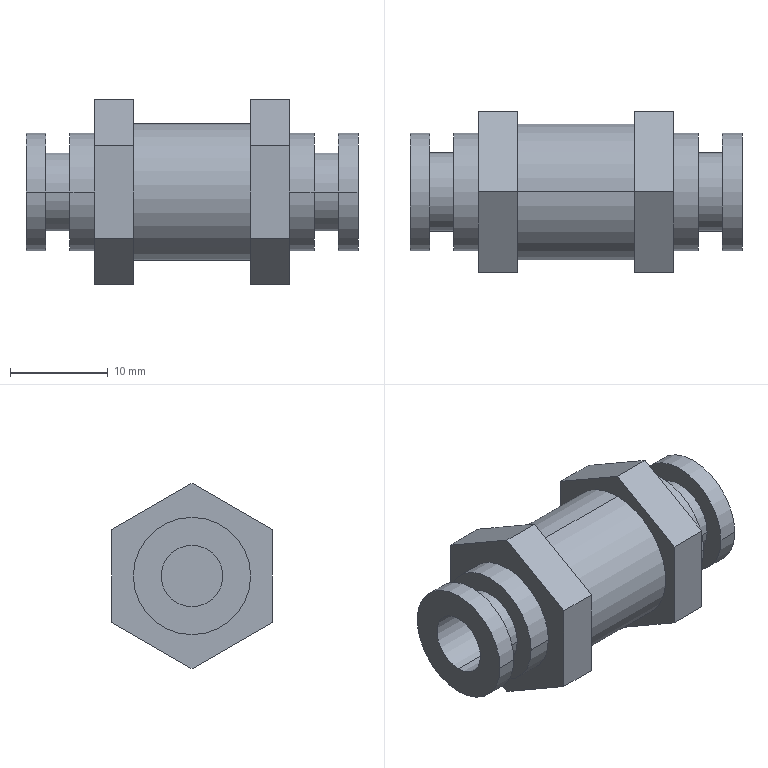Part | STEP file | QIGUANJIEKOU.stp.STEP | 1 solid | 42 faces | box 34 x 16.454 x 19 mm | volume 4306 mm3 | plane 24 | cylinder 18 | commonest cylinder face diameters 12 x8 6.3 x4 8 x4 14 x2
STEP:
#1=CARTESIAN_POINT('',(17.,0.,-3.15));
#2=VERTEX_POINT('',#1);
#3=CARTESIAN_POINT('',(17.,0.,3.15));
#4=VERTEX_POINT('',#3);
#5=CARTESIAN_POINT('',(17.,0.,0.));
#6=DIRECTION('',(1.,0.,0.));
#7=DIRECTION('',(0.,0.,-1.));
#8=AXIS2_PLACEMENT_3D('',#5,#6,#7);
#9=CIRCLE('',#8,3.15);
#10=EDGE_CURVE('',#2,#4,#9,.T.);
#11=ORIENTED_EDGE('',*,*,#10,.F.);
#12=CARTESIAN_POINT('',(17.,0.,0.));
#13=DIRECTION('',(1.,0.,0.));
#14=DIRECTION('',(0.,0.,1.));
#15=AXIS2_PLACEMENT_3D('',#12,#13,#14);
#16=CIRCLE('',#15,3.15);
#17=EDGE_CURVE('',#4,#2,#16,.T.);
#18=ORIENTED_EDGE('',*,*,#17,.F.);
#19=EDGE_LOOP('',(#11,#18));
#20=FACE_BOUND('',#19,.T.);
#21=CARTESIAN_POINT('',(17.,6.,0.));
#22=VERTEX_POINT('',#21);
#23=CARTESIAN_POINT('',(17.,-6.,0.));
#24=VERTEX_POINT('',#23);
#25=CARTESIAN_POINT('',(17.,0.,0.));
#26=DIRECTION('',(1.,0.,0.));
#27=DIRECTION('',(0.,1.,0.));
#28=AXIS2_PLACEMENT_3D('',#25,#26,#27);
#29=CIRCLE('',#28,6.);
#30=EDGE_CURVE('',#22,#24,#29,.T.);
#31=ORIENTED_EDGE('',*,*,#30,.T.);
#32=CARTESIAN_POINT('',(17.,0.,0.));
#33=DIRECTION('',(-1.,0.,0.));
#34=DIRECTION('',(0.,1.,0.));
#35=AXIS2_PLACEMENT_3D('',#32,#33,#34);
#36=CIRCLE('',#35,6.);
#37=EDGE_CURVE('',#22,#24,#36,.T.);
#38=ORIENTED_EDGE('',*,*,#37,.F.);
#39=EDGE_LOOP('',(#31,#38));
#40=FACE_OUTER_BOUND('',#39,.T.);
#41=CARTESIAN_POINT('',(17.,0.,0.));
#42=DIRECTION('',(1.,0.,0.));
#43=DIRECTION('',(0.,1.,0.));
#44=AXIS2_PLACEMENT_3D('',#41,#42,#43);
#45=PLANE('',#44);
#46=ADVANCED_FACE('',(#20,#40),#45,.T.);
#47=CARTESIAN_POINT('',(15.,6.,0.));
#48=VERTEX_POINT('',#47);
#49=CARTESIAN_POINT('',(17.,6.,0.));
#50=DIRECTION('',(-1.,0.,0.));
#51=VECTOR('',#50,1000.);
#52=LINE('',#49,#51);
#53=EDGE_CURVE('',#22,#48,#52,.T.);
#54=ORIENTED_EDGE('',*,*,#53,.F.);
#55=ORIENTED_EDGE('',*,*,#37,.T.);
#56=CARTESIAN_POINT('',(15.,-6.,0.));
#57=VERTEX_POINT('',#56);
#58=CARTESIAN_POINT('',(17.,-6.,0.));
#59=DIRECTION('',(-1.,0.,0.));
#60=VECTOR('',#59,1000.);
#61=LINE('',#58,#60);
#62=EDGE_CURVE('',#24,#57,#61,.T.);
#63=ORIENTED_EDGE('',*,*,#62,.T.);
#64=CARTESIAN_POINT('',(15.,0.,0.));
#65=DIRECTION('',(1.,0.,0.));
#66=DIRECTION('',(0.,-1.,0.));
#67=AXIS2_PLACEMENT_3D('',#64,#65,#66);
#68=CIRCLE('',#67,6.);
#69=EDGE_CURVE('',#57,#48,#68,.T.);
#70=ORIENTED_EDGE('',*,*,#69,.T.);
#71=EDGE_LOOP('',(#54,#55,#63,#70));
#72=FACE_OUTER_BOUND('',#71,.T.);
#73=CARTESIAN_POINT('',(-18.7,0.,0.));
#74=DIRECTION('',(1.,0.,0.));
#75=DIRECTION('',(0.,-1.,0.));
#76=AXIS2_PLACEMENT_3D('',#73,#74,#75);
#77=CYLINDRICAL_SURFACE('',#76,6.);
#78=ADVANCED_FACE('',(#72),#77,.T.);
#79=CARTESIAN_POINT('',(12.5,-6.,0.));
#80=VERTEX_POINT('',#79);
#81=CARTESIAN_POINT('',(10.,-6.,0.));
#82=VERTEX_POINT('',#81);
#83=CARTESIAN_POINT('',(12.5,-6.,0.));
#84=DIRECTION('',(-1.,0.,0.));
#85=VECTOR('',#84,1000.);
#86=LINE('',#83,#85);
#87=EDGE_CURVE('',#80,#82,#86,.T.);
#88=ORIENTED_EDGE('',*,*,#87,.T.);
#89=CARTESIAN_POINT('',(10.,6.,0.));
#90=VERTEX_POINT('',#89);
#91=CARTESIAN_POINT('',(10.,0.,0.));
#92=DIRECTION('',(-1.,0.,0.));
#93=DIRECTION('',(0.,1.,0.));
#94=AXIS2_PLACEMENT_3D('',#91,#92,#93);
#95=CIRCLE('',#94,6.);
#96=EDGE_CURVE('',#90,#82,#95,.T.);
#97=ORIENTED_EDGE('',*,*,#96,.F.);
#98=CARTESIAN_POINT('',(12.5,6.,0.));
#99=VERTEX_POINT('',#98);
#100=CARTESIAN_POINT('',(12.5,6.,0.));
#101=DIRECTION('',(-1.,0.,0.));
#102=VECTOR('',#101,1000.);
#103=LINE('',#100,#102);
#104=EDGE_CURVE('',#99,#90,#103,.T.);
#105=ORIENTED_EDGE('',*,*,#104,.F.);
#106=CARTESIAN_POINT('',(12.5,0.,0.));
#107=DIRECTION('',(1.,0.,0.));
#108=DIRECTION('',(0.,-1.,0.));
#109=AXIS2_PLACEMENT_3D('',#106,#107,#108);
#110=CIRCLE('',#109,6.);
#111=EDGE_CURVE('',#80,#99,#110,.T.);
#112=ORIENTED_EDGE('',*,*,#111,.F.);
#113=EDGE_LOOP('',(#88,#97,#105,#112));
#114=FACE_OUTER_BOUND('',#113,.T.);
#115=CARTESIAN_POINT('',(-18.7,0.,0.));
#116=DIRECTION('',(1.,0.,0.));
#117=DIRECTION('',(0.,-1.,0.));
#118=AXIS2_PLACEMENT_3D('',#115,#116,#117);
#119=CYLINDRICAL_SURFACE('',#118,6.);
#120=ADVANCED_FACE('',(#114),#119,.T.);
#121=CARTESIAN_POINT('',(-15.,-6.,0.));
#122=VERTEX_POINT('',#121);
#123=CARTESIAN_POINT('',(-17.,-6.,0.));
#124=VERTEX_POINT('',#123);
#125=CARTESIAN_POINT('',(-15.,-6.,0.));
#126=DIRECTION('',(-1.,0.,0.));
#127=VECTOR('',#126,1000.);
#128=LINE('',#125,#127);
#129=EDGE_CURVE('',#122,#124,#128,.T.);
#130=ORIENTED_EDGE('',*,*,#129,.T.);
#131=CARTESIAN_POINT('',(-17.,6.,0.));
#132=VERTEX_POINT('',#131);
#133=CARTESIAN_POINT('',(-17.,0.,0.));
#134=DIRECTION('',(-1.,0.,0.));
#135=DIRECTION('',(0.,1.,0.));
#136=AXIS2_PLACEMENT_3D('',#133,#134,#135);
#137=CIRCLE('',#136,6.);
#138=EDGE_CURVE('',#132,#124,#137,.T.);
#139=ORIENTED_EDGE('',*,*,#138,.F.);
#140=CARTESIAN_POINT('',(-15.,6.,0.));
#141=VERTEX_POINT('',#140);
#142=CARTESIAN_POINT('',(-15.,6.,0.));
#143=DIRECTION('',(-1.,0.,0.));
#144=VECTOR('',#143,1000.);
#145=LINE('',#142,#144);
#146=EDGE_CURVE('',#141,#132,#145,.T.);
#147=ORIENTED_EDGE('',*,*,#146,.F.);
#148=CARTESIAN_POINT('',(-15.,0.,0.));
#149=DIRECTION('',(1.,0.,0.));
#150=DIRECTION('',(0.,-1.,0.));
#151=AXIS2_PLACEMENT_3D('',#148,#149,#150);
#152=CIRCLE('',#151,6.);
#153=EDGE_CURVE('',#122,#141,#152,.T.);
#154=ORIENTED_EDGE('',*,*,#153,.F.);
#155=EDGE_LOOP('',(#130,#139,#147,#154));
#156=FACE_OUTER_BOUND('',#155,.T.);
#157=CARTESIAN_POINT('',(-18.7,0.,0.));
#158=DIRECTION('',(1.,0.,0.));
#159=DIRECTION('',(0.,-1.,0.));
#160=AXIS2_PLACEMENT_3D('',#157,#158,#159);
#161=CYLINDRICAL_SURFACE('',#160,6.);
#162=ADVANCED_FACE('',(#156),#161,.T.);
#163=CARTESIAN_POINT('',(-10.,6.,0.));
#164=VERTEX_POINT('',#163);
#165=CARTESIAN_POINT('',(-12.5,6.,0.));
#166=VERTEX_POINT('',#165);
#167=CARTESIAN_POINT('',(-10.,6.,0.));
#168=DIRECTION('',(-1.,0.,0.));
#169=VECTOR('',#168,1000.);
#170=LINE('',#167,#169);
#171=EDGE_CURVE('',#164,#166,#170,.T.);
#172=ORIENTED_EDGE('',*,*,#171,.F.);
#173=CARTESIAN_POINT('',(-10.,-6.,0.));
#174=VERTEX_POINT('',#173);
#175=CARTESIAN_POINT('',(-10.,0.,0.));
#176=DIRECTION('',(1.,0.,0.));
#177=DIRECTION('',(0.,-1.,0.));
#178=AXIS2_PLACEMENT_3D('',#175,#176,#177);
#179=CIRCLE('',#178,6.);
#180=EDGE_CURVE('',#174,#164,#179,.T.);
#181=ORIENTED_EDGE('',*,*,#180,.F.);
#182=CARTESIAN_POINT('',(-12.5,-6.,0.));
#183=VERTEX_POINT('',#182);
#184=CARTESIAN_POINT('',(-10.,-6.,0.));
#185=DIRECTION('',(-1.,0.,0.));
#186=VECTOR('',#185,1000.);
#187=LINE('',#184,#186);
#188=EDGE_CURVE('',#174,#183,#187,.T.);
#189=ORIENTED_EDGE('',*,*,#188,.T.);
#190=CARTESIAN_POINT('',(-12.5,0.,0.));
#191=DIRECTION('',(1.,0.,0.));
#192=DIRECTION('',(0.,-1.,0.));
#193=AXIS2_PLACEMENT_3D('',#190,#191,#192);
#194=CIRCLE('',#193,6.);
#195=EDGE_CURVE('',#183,#166,#194,.T.);
#196=ORIENTED_EDGE('',*,*,#195,.T.);
#197=EDGE_LOOP('',(#172,#181,#189,#196));
#198=FACE_OUTER_BOUND('',#197,.T.);
#199=CARTESIAN_POINT('',(-18.7,0.,0.));
#200=DIRECTION('',(1.,0.,0.));
#201=DIRECTION('',(0.,-1.,0.));
#202=AXIS2_PLACEMENT_3D('',#199,#200,#201);
#203=CYLINDRICAL_SURFACE('',#202,6.);
#204=ADVANCED_FACE('',(#198),#203,.T.);
#205=CARTESIAN_POINT('',(15.,-4.,0.));
#206=VERTEX_POINT('',#205);
#207=CARTESIAN_POINT('',(15.,4.,0.));
#208=VERTEX_POINT('',#207);
#209=CARTESIAN_POINT('',(15.,0.,0.));
#210=DIRECTION('',(1.,0.,0.));
#211=DIRECTION('',(0.,-1.,0.));
#212=AXIS2_PLACEMENT_3D('',#209,#210,#211);
#213=CIRCLE('',#212,4.);
#214=EDGE_CURVE('',#206,#208,#213,.T.);
#215=ORIENTED_EDGE('',*,*,#214,.T.);
#216=CARTESIAN_POINT('',(15.,0.,0.));
#217=DIRECTION('',(-1.,0.,0.));
#218=DIRECTION('',(0.,-1.,0.));
#219=AXIS2_PLACEMENT_3D('',#216,#217,#218);
#220=CIRCLE('',#219,4.);
#221=EDGE_CURVE('',#206,#208,#220,.T.);
#222=ORIENTED_EDGE('',*,*,#221,.F.);
#223=EDGE_LOOP('',(#215,#222));
#224=FACE_BOUND('',#223,.T.);
#225=ORIENTED_EDGE('',*,*,#69,.F.);
#226=CARTESIAN_POINT('',(15.,0.,0.));
#227=DIRECTION('',(1.,0.,0.));
#228=DIRECTION('',(0.,1.,0.));
#229=AXIS2_PLACEMENT_3D('',#226,#227,#228);
#230=CIRCLE('',#229,6.);
#231=EDGE_CURVE('',#48,#57,#230,.T.);
#232=ORIENTED_EDGE('',*,*,#231,.F.);
#233=EDGE_LOOP('',(#225,#232));
#234=FACE_OUTER_BOUND('',#233,.T.);
#235=CARTESIAN_POINT('',(15.,0.,0.));
#236=DIRECTION('',(1.,0.,0.));
#237=DIRECTION('',(0.,1.,0.));
#238=AXIS2_PLACEMENT_3D('',#235,#236,#237);
#239=PLANE('',#238);
#240=ADVANCED_FACE('',(#224,#234),#239,.F.);
#241=ORIENTED_EDGE('',*,*,#221,.T.);
#242=CARTESIAN_POINT('',(12.5,4.,0.));
#243=VERTEX_POINT('',#242);
#244=CARTESIAN_POINT('',(15.,4.,0.));
#245=DIRECTION('',(-1.,0.,0.));
#246=VECTOR('',#245,1000.);
#247=LINE('',#244,#246);
#248=EDGE_CURVE('',#208,#243,#247,.T.);
#249=ORIENTED_EDGE('',*,*,#248,.T.);
#250=CARTESIAN_POINT('',(12.5,-4.,0.));
#251=VERTEX_POINT('',#250);
#252=CARTESIAN_POINT('',(12.5,0.,0.));
#253=DIRECTION('',(-1.,0.,0.));
#254=DIRECTION('',(0.,-1.,0.));
#255=AXIS2_PLACEMENT_3D('',#252,#253,#254);
#256=CIRCLE('',#255,4.);
#257=EDGE_CURVE('',#251,#243,#256,.T.);
#258=ORIENTED_EDGE('',*,*,#257,.F.);
#259=CARTESIAN_POINT('',(15.,-4.,0.));
#260=DIRECTION('',(-1.,0.,0.));
#261=VECTOR('',#260,1000.);
#262=LINE('',#259,#261);
#263=EDGE_CURVE('',#206,#251,#262,.T.);
#264=ORIENTED_EDGE('',*,*,#263,.F.);
#265=EDGE_LOOP('',(#241,#249,#258,#264));
#266=FACE_OUTER_BOUND('',#265,.T.);
#267=CARTESIAN_POINT('',(12.375,0.,0.));
#268=DIRECTION('',(1.,0.,0.));
#269=DIRECTION('',(0.,-1.,0.));
#270=AXIS2_PLACEMENT_3D('',#267,#268,#269);
#271=CYLINDRICAL_SURFACE('',#270,4.);
#272=ADVANCED_FACE('',(#266),#271,.T.);
#273=CARTESIAN_POINT('',(12.5,0.,0.));
#274=DIRECTION('',(1.,0.,0.));
#275=DIRECTION('',(0.,-1.,0.));
#276=AXIS2_PLACEMENT_3D('',#273,#274,#275);
#277=CIRCLE('',#276,4.);
#278=EDGE_CURVE('',#251,#243,#277,.T.);
#279=ORIENTED_EDGE('',*,*,#278,.T.);
#280=ORIENTED_EDGE('',*,*,#248,.F.);
#281=ORIENTED_EDGE('',*,*,#214,.F.);
#282=ORIENTED_EDGE('',*,*,#263,.T.);
#283=EDGE_LOOP('',(#279,#280,#281,#282));
#284=FACE_OUTER_BOUND('',#283,.T.);
#285=CARTESIAN_POINT('',(12.375,0.,0.));
#286=DIRECTION('',(1.,0.,0.));
#287=DIRECTION('',(0.,-1.,0.));
#288=AXIS2_PLACEMENT_3D('',#285,#286,#287);
#289=CYLINDRICAL_SURFACE('',#288,4.);
#290=ADVANCED_FACE('',(#284),#289,.T.);
#291=ORIENTED_EDGE('',*,*,#257,.T.);
#292=ORIENTED_EDGE('',*,*,#278,.F.);
#293=EDGE_LOOP('',(#291,#292));
#294=FACE_BOUND('',#293,.T.);
#295=ORIENTED_EDGE('',*,*,#111,.T.);
#296=CARTESIAN_POINT('',(12.5,0.,0.));
#297=DIRECTION('',(1.,0.,0.));
#298=DIRECTION('',(0.,1.,0.));
#299=AXIS2_PLACEMENT_3D('',#296,#297,#298);
#300=CIRCLE('',#299,6.);
#301=EDGE_CURVE('',#99,#80,#300,.T.);
#302=ORIENTED_EDGE('',*,*,#301,.T.);
#303=EDGE_LOOP('',(#295,#302));
#304=FACE_OUTER_BOUND('',#303,.T.);
#305=CARTESIAN_POINT('',(12.5,0.,0.));
#306=DIRECTION('',(1.,0.,0.));
#307=DIRECTION('',(0.,1.,0.));
#308=AXIS2_PLACEMENT_3D('',#305,#306,#307);
#309=PLANE('',#308);
#310=ADVANCED_FACE('',(#294,#304),#309,.T.);
#311=ORIENTED_EDGE('',*,*,#62,.F.);
#312=ORIENTED_EDGE('',*,*,#30,.F.);
#313=ORIENTED_EDGE('',*,*,#53,.T.);
#314=ORIENTED_EDGE('',*,*,#231,.T.);
#315=EDGE_LOOP('',(#311,#312,#313,#314));
#316=FACE_OUTER_BOUND('',#315,.T.);
#317=CARTESIAN_POINT('',(-18.7,0.,0.));
#318=DIRECTION('',(1.,0.,0.));
#319=DIRECTION('',(0.,-1.,0.));
#320=AXIS2_PLACEMENT_3D('',#317,#318,#319);
#321=CYLINDRICAL_SURFACE('',#320,6.);
#322=ADVANCED_FACE('',(#316),#321,.T.);
#323=ORIENTED_EDGE('',*,*,#104,.T.);
#324=CARTESIAN_POINT('',(10.,0.,0.));
#325=DIRECTION('',(-1.,0.,0.));
#326=DIRECTION('',(0.,-1.,0.));
#327=AXIS2_PLACEMENT_3D('',#324,#325,#326);
#328=CIRCLE('',#327,6.);
#329=EDGE_CURVE('',#82,#90,#328,.T.);
#330=ORIENTED_EDGE('',*,*,#329,.F.);
#331=ORIENTED_EDGE('',*,*,#87,.F.);
#332=ORIENTED_EDGE('',*,*,#301,.F.);
#333=EDGE_LOOP('',(#323,#330,#331,#332));
#334=FACE_OUTER_BOUND('',#333,.T.);
#335=CARTESIAN_POINT('',(-18.7,0.,0.));
#336=DIRECTION('',(1.,0.,0.));
#337=DIRECTION('',(0.,-1.,0.));
#338=AXIS2_PLACEMENT_3D('',#335,#336,#337);
#339=CYLINDRICAL_SURFACE('',#338,6.);
#340=ADVANCED_FACE('',(#334),#339,.T.);
#341=ORIENTED_EDGE('',*,*,#146,.T.);
#342=CARTESIAN_POINT('',(-17.,0.,0.));
#343=DIRECTION('',(1.,0.,0.));
#344=DIRECTION('',(0.,1.,0.));
#345=AXIS2_PLACEMENT_3D('',#342,#343,#344);
#346=CIRCLE('',#345,6.);
#347=EDGE_CURVE('',#132,#124,#346,.T.);
#348=ORIENTED_EDGE('',*,*,#347,.T.);
#349=ORIENTED_EDGE('',*,*,#129,.F.);
#350=CARTESIAN_POINT('',(-15.,0.,0.));
#351=DIRECTION('',(1.,0.,0.));
#352=DIRECTION('',(0.,1.,0.));
#353=AXIS2_PLACEMENT_3D('',#350,#351,#352);
#354=CIRCLE('',#353,6.);
#355=EDGE_CURVE('',#141,#122,#354,.T.);
#356=ORIENTED_EDGE('',*,*,#355,.F.);
#357=EDGE_LOOP('',(#341,#348,#349,#356));
#358=FACE_OUTER_BOUND('',#357,.T.);
#359=CARTESIAN_POINT('',(-18.7,0.,0.));
#360=DIRECTION('',(1.,0.,0.));
#361=DIRECTION('',(0.,-1.,0.));
#362=AXIS2_PLACEMENT_3D('',#359,#360,#361);
#363=CYLINDRICAL_SURFACE('',#362,6.);
#364=ADVANCED_FACE('',(#358),#363,.T.);
#365=ORIENTED_EDGE('',*,*,#188,.F.);
#366=CARTESIAN_POINT('',(-10.,0.,0.));
#367=DIRECTION('',(1.,0.,0.));
#368=DIRECTION('',(0.,1.,0.));
#369=AXIS2_PLACEMENT_3D('',#366,#367,#368);
#370=CIRCLE('',#369,6.);
#371=EDGE_CURVE('',#164,#174,#370,.T.);
#372=ORIENTED_EDGE('',*,*,#371,.F.);
#373=ORIENTED_EDGE('',*,*,#171,.T.);
#374=CARTESIAN_POINT('',(-12.5,0.,0.));
#375=DIRECTION('',(1.,0.,0.));
#376=DIRECTION('',(0.,1.,0.));
#377=AXIS2_PLACEMENT_3D('',#374,#375,#376);
#378=CIRCLE('',#377,6.);
#379=EDGE_CURVE('',#166,#183,#378,.T.);
#380=ORIENTED_EDGE('',*,*,#379,.T.);
#381=EDGE_LOOP('',(#365,#372,#373,#380));
#382=FACE_OUTER_BOUND('',#381,.T.);
#383=CARTESIAN_POINT('',(-18.7,0.,0.));
#384=DIRECTION('',(1.,0.,0.));
#385=DIRECTION('',(0.,-1.,0.));
#386=AXIS2_PLACEMENT_3D('',#383,#384,#385);
#387=CYLINDRICAL_SURFACE('',#386,6.);
#388=ADVANCED_FACE('',(#382),#387,.T.);
#389=ORIENTED_EDGE('',*,*,#96,.T.);
#390=ORIENTED_EDGE('',*,*,#329,.T.);
#391=EDGE_LOOP('',(#389,#390));
#392=FACE_BOUND('',#391,.T.);
#393=CARTESIAN_POINT('',(10.,0.,-9.5));
#394=VERTEX_POINT('',#393);
#395=CARTESIAN_POINT('',(10.,-8.227,-4.75));
#396=VERTEX_POINT('',#395);
#397=CARTESIAN_POINT('',(10.,0.,-9.5));
#398=DIRECTION('',(0.,-0.866,0.5));
#399=VECTOR('',#398,1000.);
#400=LINE('',#397,#399);
#401=EDGE_CURVE('',#394,#396,#400,.T.);
#402=ORIENTED_EDGE('',*,*,#401,.F.);
#403=CARTESIAN_POINT('',(10.,8.227,-4.75));
#404=VERTEX_POINT('',#403);
#405=CARTESIAN_POINT('',(10.,8.227,-4.75));
#406=DIRECTION('',(0.,-0.866,-0.5));
#407=VECTOR('',#406,1000.);
#408=LINE('',#405,#407);
#409=EDGE_CURVE('',#404,#394,#408,.T.);
#410=ORIENTED_EDGE('',*,*,#409,.F.);
#411=CARTESIAN_POINT('',(10.,8.227,4.75));
#412=VERTEX_POINT('',#411);
#413=CARTESIAN_POINT('',(10.,8.227,4.75));
#414=DIRECTION('',(0.,0.,-1.));
#415=VECTOR('',#414,1000.);
#416=LINE('',#413,#415);
#417=EDGE_CURVE('',#412,#404,#416,.T.);
#418=ORIENTED_EDGE('',*,*,#417,.F.);
#419=CARTESIAN_POINT('',(10.,0.,9.5));
#420=VERTEX_POINT('',#419);
#421=CARTESIAN_POINT('',(10.,0.,9.5));
#422=DIRECTION('',(0.,0.866,-0.5));
#423=VECTOR('',#422,1000.);
#424=LINE('',#421,#423);
#425=EDGE_CURVE('',#420,#412,#424,.T.);
#426=ORIENTED_EDGE('',*,*,#425,.F.);
#427=CARTESIAN_POINT('',(10.,-8.227,4.75));
#428=VERTEX_POINT('',#427);
#429=CARTESIAN_POINT('',(10.,-8.227,4.75));
#430=DIRECTION('',(0.,0.866,0.5));
#431=VECTOR('',#430,1000.);
#432=LINE('',#429,#431);
#433=EDGE_CURVE('',#428,#420,#432,.T.);
#434=ORIENTED_EDGE('',*,*,#433,.F.);
#435=CARTESIAN_POINT('',(10.,-8.227,-4.75));
#436=DIRECTION('',(0.,0.,1.));
#437=VECTOR('',#436,1000.);
#438=LINE('',#435,#437);
#439=EDGE_CURVE('',#396,#428,#438,.T.);
#440=ORIENTED_EDGE('',*,*,#439,.F.);
#441=EDGE_LOOP('',(#402,#410,#418,#426,#434,#440));
#442=FACE_OUTER_BOUND('',#441,.T.);
#443=CARTESIAN_POINT('',(10.,0.,0.));
#444=DIRECTION('',(1.,0.,0.));
#445=DIRECTION('',(0.,1.,0.));
#446=AXIS2_PLACEMENT_3D('',#443,#444,#445);
#447=PLANE('',#446);
#448=ADVANCED_FACE('',(#392,#442),#447,.T.);
#449=CARTESIAN_POINT('',(6.,-8.227,4.75));
#450=VERTEX_POINT('',#449);
#451=CARTESIAN_POINT('',(10.,-8.227,4.75));
#452=DIRECTION('',(-1.,0.,0.));
#453=VECTOR('',#452,1000.);
#454=LINE('',#451,#453);
#455=EDGE_CURVE('',#428,#450,#454,.T.);
#456=ORIENTED_EDGE('',*,*,#455,.T.);
#457=CARTESIAN_POINT('',(6.,-8.227,-4.75));
#458=VERTEX_POINT('',#457);
#459=CARTESIAN_POINT('',(6.,-8.227,-4.75));
#460=DIRECTION('',(0.,0.,1.));
#461=VECTOR('',#460,1000.);
#462=LINE('',#459,#461);
#463=EDGE_CURVE('',#458,#450,#462,.T.);
#464=ORIENTED_EDGE('',*,*,#463,.F.);
#465=CARTESIAN_POINT('',(10.,-8.227,-4.75));
#466=DIRECTION('',(-1.,0.,0.));
#467=VECTOR('',#466,1000.);
#468=LINE('',#465,#467);
#469=EDGE_CURVE('',#396,#458,#468,.T.);
#470=ORIENTED_EDGE('',*,*,#469,.F.);
#471=ORIENTED_EDGE('',*,*,#439,.T.);
#472=EDGE_LOOP('',(#456,#464,#470,#471));
#473=FACE_OUTER_BOUND('',#472,.T.);
#474=CARTESIAN_POINT('',(10.,-8.227,-4.75));
#475=DIRECTION('',(0.,1.,0.));
#476=DIRECTION('',(1.,0.,0.));
#477=AXIS2_PLACEMENT_3D('',#474,#475,#476);
#478=PLANE('',#477);
#479=ADVANCED_FACE('',(#473),#478,.F.);
#480=CARTESIAN_POINT('',(-6.,-8.227,4.75));
#481=VERTEX_POINT('',#480);
#482=CARTESIAN_POINT('',(-10.,-8.227,4.75));
#483=VERTEX_POINT('',#482);
#484=CARTESIAN_POINT('',(-6.,-8.227,4.75));
#485=DIRECTION('',(-1.,0.,0.));
#486=VECTOR('',#485,1000.);
#487=LINE('',#484,#486);
#488=EDGE_CURVE('',#481,#483,#487,.T.);
#489=ORIENTED_EDGE('',*,*,#488,.T.);
#490=CARTESIAN_POINT('',(-10.,-8.227,-4.75));
#491=VERTEX_POINT('',#490);
#492=CARTESIAN_POINT('',(-10.,-8.227,-4.75));
#493=DIRECTION('',(0.,0.,1.));
#494=VECTOR('',#493,1000.);
#495=LINE('',#492,#494);
#496=EDGE_CURVE('',#491,#483,#495,.T.);
#497=ORIENTED_EDGE('',*,*,#496,.F.);
#498=CARTESIAN_POINT('',(-6.,-8.227,-4.75));
#499=VERTEX_POINT('',#498);
#500=CARTESIAN_POINT('',(-6.,-8.227,-4.75));
#501=DIRECTION('',(-1.,0.,0.));
#502=VECTOR('',#501,1000.);
#503=LINE('',#500,#502);
#504=EDGE_CURVE('',#499,#491,#503,.T.);
#505=ORIENTED_EDGE('',*,*,#504,.F.);
#506=CARTESIAN_POINT('',(-6.,-8.227,-4.75));
#507=DIRECTION('',(0.,0.,1.));
#508=VECTOR('',#507,1000.);
#509=LINE('',#506,#508);
#510=EDGE_CURVE('',#499,#481,#509,.T.);
#511=ORIENTED_EDGE('',*,*,#510,.T.);
#512=EDGE_LOOP('',(#489,#497,#505,#511));
#513=FACE_OUTER_BOUND('',#512,.T.);
#514=CARTESIAN_POINT('',(10.,-8.227,-4.75));
#515=DIRECTION('',(0.,1.,0.));
#516=DIRECTION('',(1.,0.,0.));
#517=AXIS2_PLACEMENT_3D('',#514,#515,#516);
#518=PLANE('',#517);
#519=ADVANCED_FACE('',(#513),#518,.F.);
#520=ORIENTED_EDGE('',*,*,#469,.T.);
#521=CARTESIAN_POINT('',(6.,0.,-9.5));
#522=VERTEX_POINT('',#521);
#523=CARTESIAN_POINT('',(6.,0.,-9.5));
#524=DIRECTION('',(0.,-0.866,0.5));
#525=VECTOR('',#524,1000.);
#526=LINE('',#523,#525);
#527=EDGE_CURVE('',#522,#458,#526,.T.);
#528=ORIENTED_EDGE('',*,*,#527,.F.);
#529=CARTESIAN_POINT('',(10.,0.,-9.5));
#530=DIRECTION('',(-1.,0.,0.));
#531=VECTOR('',#530,1000.);
#532=LINE('',#529,#531);
#533=EDGE_CURVE('',#394,#522,#532,.T.);
#534=ORIENTED_EDGE('',*,*,#533,.F.);
#535=ORIENTED_EDGE('',*,*,#401,.T.);
#536=EDGE_LOOP('',(#520,#528,#534,#535));
#537=FACE_OUTER_BOUND('',#536,.T.);
#538=CARTESIAN_POINT('',(10.,0.,-9.5));
#539=DIRECTION('',(0.,0.5,0.866));
#540=DIRECTION('',(1.,0.,0.));
#541=AXIS2_PLACEMENT_3D('',#538,#539,#540);
#542=PLANE('',#541);
#543=ADVANCED_FACE('',(#537),#542,.F.);
#544=ORIENTED_EDGE('',*,*,#504,.T.);
#545=CARTESIAN_POINT('',(-10.,0.,-9.5));
#546=VERTEX_POINT('',#545);
#547=CARTESIAN_POINT('',(-10.,0.,-9.5));
#548=DIRECTION('',(0.,-0.866,0.5));
#549=VECTOR('',#548,1000.);
#550=LINE('',#547,#549);
#551=EDGE_CURVE('',#546,#491,#550,.T.);
#552=ORIENTED_EDGE('',*,*,#551,.F.);
#553=CARTESIAN_POINT('',(-6.,0.,-9.5));
#554=VERTEX_POINT('',#553);
#555=CARTESIAN_POINT('',(-6.,0.,-9.5));
#556=DIRECTION('',(-1.,0.,0.));
#557=VECTOR('',#556,1000.);
#558=LINE('',#555,#557);
#559=EDGE_CURVE('',#554,#546,#558,.T.);
#560=ORIENTED_EDGE('',*,*,#559,.F.);
#561=CARTESIAN_POINT('',(-6.,0.,-9.5));
#562=DIRECTION('',(0.,-0.866,0.5));
#563=VECTOR('',#562,1000.);
#564=LINE('',#561,#563);
#565=EDGE_CURVE('',#554,#499,#564,.T.);
#566=ORIENTED_EDGE('',*,*,#565,.T.);
#567=EDGE_LOOP('',(#544,#552,#560,#566));
#568=FACE_OUTER_BOUND('',#567,.T.);
#569=CARTESIAN_POINT('',(10.,0.,-9.5));
#570=DIRECTION('',(0.,0.5,0.866));
#571=DIRECTION('',(1.,0.,0.));
#572=AXIS2_PLACEMENT_3D('',#569,#570,#571);
#573=PLANE('',#572);
#574=ADVANCED_FACE('',(#568),#573,.F.);
#575=ORIENTED_EDGE('',*,*,#533,.T.);
#576=CARTESIAN_POINT('',(6.,8.227,-4.75));
#577=VERTEX_POINT('',#576);
#578=CARTESIAN_POINT('',(6.,8.227,-4.75));
#579=DIRECTION('',(0.,-0.866,-0.5));
#580=VECTOR('',#579,1000.);
#581=LINE('',#578,#580);
#582=EDGE_CURVE('',#577,#522,#581,.T.);
#583=ORIENTED_EDGE('',*,*,#582,.F.);
#584=CARTESIAN_POINT('',(10.,8.227,-4.75));
#585=DIRECTION('',(-1.,0.,0.));
#586=VECTOR('',#585,1000.);
#587=LINE('',#584,#586);
#588=EDGE_CURVE('',#404,#577,#587,.T.);
#589=ORIENTED_EDGE('',*,*,#588,.F.);
#590=ORIENTED_EDGE('',*,*,#409,.T.);
#591=EDGE_LOOP('',(#575,#583,#589,#590));
#592=FACE_OUTER_BOUND('',#591,.T.);
#593=CARTESIAN_POINT('',(10.,8.227,-4.75));
#594=DIRECTION('',(0.,-0.5,0.866));
#595=DIRECTION('',(-1.,0.,0.));
#596=AXIS2_PLACEMENT_3D('',#593,#594,#595);
#597=PLANE('',#596);
#598=ADVANCED_FACE('',(#592),#597,.F.);
#599=ORIENTED_EDGE('',*,*,#559,.T.);
#600=CARTESIAN_POINT('',(-10.,8.227,-4.75));
#601=VERTEX_POINT('',#600);
#602=CARTESIAN_POINT('',(-10.,8.227,-4.75));
#603=DIRECTION('',(0.,-0.866,-0.5));
#604=VECTOR('',#603,1000.);
#605=LINE('',#602,#604);
#606=EDGE_CURVE('',#601,#546,#605,.T.);
#607=ORIENTED_EDGE('',*,*,#606,.F.);
#608=CARTESIAN_POINT('',(-6.,8.227,-4.75));
#609=VERTEX_POINT('',#608);
#610=CARTESIAN_POINT('',(-6.,8.227,-4.75));
#611=DIRECTION('',(-1.,0.,0.));
#612=VECTOR('',#611,1000.);
#613=LINE('',#610,#612);
#614=EDGE_CURVE('',#609,#601,#613,.T.);
#615=ORIENTED_EDGE('',*,*,#614,.F.);
#616=CARTESIAN_POINT('',(-6.,8.227,-4.75));
#617=DIRECTION('',(0.,-0.866,-0.5));
#618=VECTOR('',#617,1000.);
#619=LINE('',#616,#618);
#620=EDGE_CURVE('',#609,#554,#619,.T.);
#621=ORIENTED_EDGE('',*,*,#620,.T.);
#622=EDGE_LOOP('',(#599,#607,#615,#621));
#623=FACE_OUTER_BOUND('',#622,.T.);
#624=CARTESIAN_POINT('',(10.,8.227,-4.75));
#625=DIRECTION('',(0.,-0.5,0.866));
#626=DIRECTION('',(-1.,0.,0.));
#627=AXIS2_PLACEMENT_3D('',#624,#625,#626);
#628=PLANE('',#627);
#629=ADVANCED_FACE('',(#623),#628,.F.);
#630=ORIENTED_EDGE('',*,*,#588,.T.);
#631=CARTESIAN_POINT('',(6.,8.227,4.75));
#632=VERTEX_POINT('',#631);
#633=CARTESIAN_POINT('',(6.,8.227,4.75));
#634=DIRECTION('',(0.,0.,-1.));
#635=VECTOR('',#634,1000.);
#636=LINE('',#633,#635);
#637=EDGE_CURVE('',#632,#577,#636,.T.);
#638=ORIENTED_EDGE('',*,*,#637,.F.);
#639=CARTESIAN_POINT('',(10.,8.227,4.75));
#640=DIRECTION('',(-1.,0.,0.));
#641=VECTOR('',#640,1000.);
#642=LINE('',#639,#641);
#643=EDGE_CURVE('',#412,#632,#642,.T.);
#644=ORIENTED_EDGE('',*,*,#643,.F.);
#645=ORIENTED_EDGE('',*,*,#417,.T.);
#646=EDGE_LOOP('',(#630,#638,#644,#645));
#647=FACE_OUTER_BOUND('',#646,.T.);
#648=CARTESIAN_POINT('',(10.,8.227,4.75));
#649=DIRECTION('',(0.,-1.,0.));
#650=DIRECTION('',(0.,0.,-1.));
#651=AXIS2_PLACEMENT_3D('',#648,#649,#650);
#652=PLANE('',#651);
#653=ADVANCED_FACE('',(#647),#652,.F.);
#654=ORIENTED_EDGE('',*,*,#614,.T.);
#655=CARTESIAN_POINT('',(-10.,8.227,4.75));
#656=VERTEX_POINT('',#655);
#657=CARTESIAN_POINT('',(-10.,8.227,4.75));
#658=DIRECTION('',(0.,0.,-1.));
#659=VECTOR('',#658,1000.);
#660=LINE('',#657,#659);
#661=EDGE_CURVE('',#656,#601,#660,.T.);
#662=ORIENTED_EDGE('',*,*,#661,.F.);
#663=CARTESIAN_POINT('',(-6.,8.227,4.75));
#664=VERTEX_POINT('',#663);
#665=CARTESIAN_POINT('',(-6.,8.227,4.75));
#666=DIRECTION('',(-1.,0.,0.));
#667=VECTOR('',#666,1000.);
#668=LINE('',#665,#667);
#669=EDGE_CURVE('',#664,#656,#668,.T.);
#670=ORIENTED_EDGE('',*,*,#669,.F.);
#671=CARTESIAN_POINT('',(-6.,8.227,4.75));
#672=DIRECTION('',(0.,0.,-1.));
#673=VECTOR('',#672,1000.);
#674=LINE('',#671,#673);
#675=EDGE_CURVE('',#664,#609,#674,.T.);
#676=ORIENTED_EDGE('',*,*,#675,.T.);
#677=EDGE_LOOP('',(#654,#662,#670,#676));
#678=FACE_OUTER_BOUND('',#677,.T.);
#679=CARTESIAN_POINT('',(10.,8.227,4.75));
#680=DIRECTION('',(0.,-1.,0.));
#681=DIRECTION('',(0.,0.,-1.));
#682=AXIS2_PLACEMENT_3D('',#679,#680,#681);
#683=PLANE('',#682);
#684=ADVANCED_FACE('',(#678),#683,.F.);
#685=ORIENTED_EDGE('',*,*,#643,.T.);
#686=CARTESIAN_POINT('',(6.,0.,9.5));
#687=VERTEX_POINT('',#686);
#688=CARTESIAN_POINT('',(6.,0.,9.5));
#689=DIRECTION('',(0.,0.866,-0.5));
#690=VECTOR('',#689,1000.);
#691=LINE('',#688,#690);
#692=EDGE_CURVE('',#687,#632,#691,.T.);
#693=ORIENTED_EDGE('',*,*,#692,.F.);
#694=CARTESIAN_POINT('',(10.,0.,9.5));
#695=DIRECTION('',(-1.,0.,0.));
#696=VECTOR('',#695,1000.);
#697=LINE('',#694,#696);
#698=EDGE_CURVE('',#420,#687,#697,.T.);
#699=ORIENTED_EDGE('',*,*,#698,.F.);
#700=ORIENTED_EDGE('',*,*,#425,.T.);
#701=EDGE_LOOP('',(#685,#693,#699,#700));
#702=FACE_OUTER_BOUND('',#701,.T.);
#703=CARTESIAN_POINT('',(10.,0.,9.5));
#704=DIRECTION('',(0.,-0.5,-0.866));
#705=DIRECTION('',(0.,-0.866,0.5));
#706=AXIS2_PLACEMENT_3D('',#703,#704,#705);
#707=PLANE('',#706);
#708=ADVANCED_FACE('',(#702),#707,.F.);
#709=ORIENTED_EDGE('',*,*,#669,.T.);
#710=CARTESIAN_POINT('',(-10.,0.,9.5));
#711=VERTEX_POINT('',#710);
#712=CARTESIAN_POINT('',(-10.,0.,9.5));
#713=DIRECTION('',(0.,0.866,-0.5));
#714=VECTOR('',#713,1000.);
#715=LINE('',#712,#714);
#716=EDGE_CURVE('',#711,#656,#715,.T.);
#717=ORIENTED_EDGE('',*,*,#716,.F.);
#718=CARTESIAN_POINT('',(-6.,0.,9.5));
#719=VERTEX_POINT('',#718);
#720=CARTESIAN_POINT('',(-6.,0.,9.5));
#721=DIRECTION('',(-1.,0.,0.));
#722=VECTOR('',#721,1000.);
#723=LINE('',#720,#722);
#724=EDGE_CURVE('',#719,#711,#723,.T.);
#725=ORIENTED_EDGE('',*,*,#724,.F.);
#726=CARTESIAN_POINT('',(-6.,0.,9.5));
#727=DIRECTION('',(0.,0.866,-0.5));
#728=VECTOR('',#727,1000.);
#729=LINE('',#726,#728);
#730=EDGE_CURVE('',#719,#664,#729,.T.);
#731=ORIENTED_EDGE('',*,*,#730,.T.);
#732=EDGE_LOOP('',(#709,#717,#725,#731));
#733=FACE_OUTER_BOUND('',#732,.T.);
#734=CARTESIAN_POINT('',(10.,0.,9.5));
#735=DIRECTION('',(0.,-0.5,-0.866));
#736=DIRECTION('',(0.,-0.866,0.5));
#737=AXIS2_PLACEMENT_3D('',#734,#735,#736);
#738=PLANE('',#737);
#739=ADVANCED_FACE('',(#733),#738,.F.);
#740=ORIENTED_EDGE('',*,*,#698,.T.);
#741=CARTESIAN_POINT('',(6.,-8.227,4.75));
#742=DIRECTION('',(0.,0.866,0.5));
#743=VECTOR('',#742,1000.);
#744=LINE('',#741,#743);
#745=EDGE_CURVE('',#450,#687,#744,.T.);
#746=ORIENTED_EDGE('',*,*,#745,.F.);
#747=ORIENTED_EDGE('',*,*,#455,.F.);
#748=ORIENTED_EDGE('',*,*,#433,.T.);
#749=EDGE_LOOP('',(#740,#746,#747,#748));
#750=FACE_OUTER_BOUND('',#749,.T.);
#751=CARTESIAN_POINT('',(10.,-8.227,4.75));
#752=DIRECTION('',(0.,0.5,-0.866));
#753=DIRECTION('',(-1.,0.,0.));
#754=AXIS2_PLACEMENT_3D('',#751,#752,#753);
#755=PLANE('',#754);
#756=ADVANCED_FACE('',(#750),#755,.F.);
#757=ORIENTED_EDGE('',*,*,#724,.T.);
#758=CARTESIAN_POINT('',(-10.,-8.227,4.75));
#759=DIRECTION('',(0.,0.866,0.5));
#760=VECTOR('',#759,1000.);
#761=LINE('',#758,#760);
#762=EDGE_CURVE('',#483,#711,#761,.T.);
#763=ORIENTED_EDGE('',*,*,#762,.F.);
#764=ORIENTED_EDGE('',*,*,#488,.F.);
#765=CARTESIAN_POINT('',(-6.,-8.227,4.75));
#766=DIRECTION('',(0.,0.866,0.5));
#767=VECTOR('',#766,1000.);
#768=LINE('',#765,#767);
#769=EDGE_CURVE('',#481,#719,#768,.T.);
#770=ORIENTED_EDGE('',*,*,#769,.T.);
#771=EDGE_LOOP('',(#757,#763,#764,#770));
#772=FACE_OUTER_BOUND('',#771,.T.);
#773=CARTESIAN_POINT('',(10.,-8.227,4.75));
#774=DIRECTION('',(0.,0.5,-0.866));
#775=DIRECTION('',(-1.,0.,0.));
#776=AXIS2_PLACEMENT_3D('',#773,#774,#775);
#777=PLANE('',#776);
#778=ADVANCED_FACE('',(#772),#777,.F.);
#779=CARTESIAN_POINT('',(6.,0.,-7.));
#780=VERTEX_POINT('',#779);
#781=CARTESIAN_POINT('',(6.,0.,7.));
#782=VERTEX_POINT('',#781);
#783=CARTESIAN_POINT('',(6.,0.,0.));
#784=DIRECTION('',(1.,0.,0.));
#785=DIRECTION('',(0.,0.,-1.));
#786=AXIS2_PLACEMENT_3D('',#783,#784,#785);
#787=CIRCLE('',#786,7.);
#788=EDGE_CURVE('',#780,#782,#787,.T.);
#789=ORIENTED_EDGE('',*,*,#788,.T.);
#790=CARTESIAN_POINT('',(6.,0.,0.));
#791=DIRECTION('',(1.,0.,0.));
#792=DIRECTION('',(0.,0.,1.));
#793=AXIS2_PLACEMENT_3D('',#790,#791,#792);
#794=CIRCLE('',#793,7.);
#795=EDGE_CURVE('',#782,#780,#794,.T.);
#796=ORIENTED_EDGE('',*,*,#795,.T.);
#797=EDGE_LOOP('',(#789,#796));
#798=FACE_BOUND('',#797,.T.);
#799=ORIENTED_EDGE('',*,*,#745,.T.);
#800=ORIENTED_EDGE('',*,*,#692,.T.);
#801=ORIENTED_EDGE('',*,*,#637,.T.);
#802=ORIENTED_EDGE('',*,*,#582,.T.);
#803=ORIENTED_EDGE('',*,*,#527,.T.);
#804=ORIENTED_EDGE('',*,*,#463,.T.);
#805=EDGE_LOOP('',(#799,#800,#801,#802,#803,#804));
#806=FACE_OUTER_BOUND('',#805,.T.);
#807=CARTESIAN_POINT('',(6.,0.,0.));
#808=DIRECTION('',(1.,0.,0.));
#809=DIRECTION('',(0.,1.,0.));
#810=AXIS2_PLACEMENT_3D('',#807,#808,#809);
#811=PLANE('',#810);
#812=ADVANCED_FACE('',(#798,#806),#811,.F.);
#813=CARTESIAN_POINT('',(-6.,0.,7.));
#814=VERTEX_POINT('',#813);
#815=CARTESIAN_POINT('',(-6.,0.,7.));
#816=DIRECTION('',(1.,0.,0.));
#817=VECTOR('',#816,1000.);
#818=LINE('',#815,#817);
#819=EDGE_CURVE('',#814,#782,#818,.T.);
#820=ORIENTED_EDGE('',*,*,#819,.F.);
#821=CARTESIAN_POINT('',(-6.,0.,-7.));
#822=VERTEX_POINT('',#821);
#823=CARTESIAN_POINT('',(-6.,0.,0.));
#824=DIRECTION('',(1.,0.,0.));
#825=DIRECTION('',(0.,0.,1.));
#826=AXIS2_PLACEMENT_3D('',#823,#824,#825);
#827=CIRCLE('',#826,7.);
#828=EDGE_CURVE('',#814,#822,#827,.T.);
#829=ORIENTED_EDGE('',*,*,#828,.T.);
#830=CARTESIAN_POINT('',(-6.,0.,-7.));
#831=DIRECTION('',(1.,0.,0.));
#832=VECTOR('',#831,1000.);
#833=LINE('',#830,#832);
#834=EDGE_CURVE('',#822,#780,#833,.T.);
#835=ORIENTED_EDGE('',*,*,#834,.T.);
#836=ORIENTED_EDGE('',*,*,#795,.F.);
#837=EDGE_LOOP('',(#820,#829,#835,#836));
#838=FACE_OUTER_BOUND('',#837,.T.);
#839=CARTESIAN_POINT('',(-6.,0.,0.));
#840=DIRECTION('',(1.,0.,0.));
#841=DIRECTION('',(0.,0.,1.));
#842=AXIS2_PLACEMENT_3D('',#839,#840,#841);
#843=CYLINDRICAL_SURFACE('',#842,7.);
#844=ADVANCED_FACE('',(#838),#843,.T.);
#845=ORIENTED_EDGE('',*,*,#834,.F.);
#846=CARTESIAN_POINT('',(-6.,0.,0.));
#847=DIRECTION('',(1.,0.,0.));
#848=DIRECTION('',(0.,0.,-1.));
#849=AXIS2_PLACEMENT_3D('',#846,#847,#848);
#850=CIRCLE('',#849,7.);
#851=EDGE_CURVE('',#822,#814,#850,.T.);
#852=ORIENTED_EDGE('',*,*,#851,.T.);
#853=ORIENTED_EDGE('',*,*,#819,.T.);
#854=ORIENTED_EDGE('',*,*,#788,.F.);
#855=EDGE_LOOP('',(#845,#852,#853,#854));
#856=FACE_OUTER_BOUND('',#855,.T.);
#857=CARTESIAN_POINT('',(-6.,0.,0.));
#858=DIRECTION('',(1.,0.,0.));
#859=DIRECTION('',(0.,0.,1.));
#860=AXIS2_PLACEMENT_3D('',#857,#858,#859);
#861=CYLINDRICAL_SURFACE('',#860,7.);
#862=ADVANCED_FACE('',(#856),#861,.T.);
#863=ORIENTED_EDGE('',*,*,#851,.F.);
#864=ORIENTED_EDGE('',*,*,#828,.F.);
#865=EDGE_LOOP('',(#863,#864));
#866=FACE_BOUND('',#865,.T.);
#867=ORIENTED_EDGE('',*,*,#565,.F.);
#868=ORIENTED_EDGE('',*,*,#620,.F.);
#869=ORIENTED_EDGE('',*,*,#675,.F.);
#870=ORIENTED_EDGE('',*,*,#730,.F.);
#871=ORIENTED_EDGE('',*,*,#769,.F.);
#872=ORIENTED_EDGE('',*,*,#510,.F.);
#873=EDGE_LOOP('',(#867,#868,#869,#870,#871,#872));
#874=FACE_OUTER_BOUND('',#873,.T.);
#875=CARTESIAN_POINT('',(-6.,0.,0.));
#876=DIRECTION('',(1.,0.,0.));
#877=DIRECTION('',(0.,1.,0.));
#878=AXIS2_PLACEMENT_3D('',#875,#876,#877);
#879=PLANE('',#878);
#880=ADVANCED_FACE('',(#866,#874),#879,.T.);
#881=ORIENTED_EDGE('',*,*,#180,.T.);
#882=ORIENTED_EDGE('',*,*,#371,.T.);
#883=EDGE_LOOP('',(#881,#882));
#884=FACE_BOUND('',#883,.T.);
#885=ORIENTED_EDGE('',*,*,#762,.T.);
#886=ORIENTED_EDGE('',*,*,#716,.T.);
#887=ORIENTED_EDGE('',*,*,#661,.T.);
#888=ORIENTED_EDGE('',*,*,#606,.T.);
#889=ORIENTED_EDGE('',*,*,#551,.T.);
#890=ORIENTED_EDGE('',*,*,#496,.T.);
#891=EDGE_LOOP('',(#885,#886,#887,#888,#889,#890));
#892=FACE_OUTER_BOUND('',#891,.T.);
#893=CARTESIAN_POINT('',(-10.,0.,0.));
#894=DIRECTION('',(1.,0.,0.));
#895=DIRECTION('',(0.,1.,0.));
#896=AXIS2_PLACEMENT_3D('',#893,#894,#895);
#897=PLANE('',#896);
#898=ADVANCED_FACE('',(#884,#892),#897,.F.);
#899=CARTESIAN_POINT('',(-15.,-4.,0.));
#900=VERTEX_POINT('',#899);
#901=CARTESIAN_POINT('',(-15.,4.,0.));
#902=VERTEX_POINT('',#901);
#903=CARTESIAN_POINT('',(-15.,0.,0.));
#904=DIRECTION('',(1.,0.,0.));
#905=DIRECTION('',(0.,-1.,0.));
#906=AXIS2_PLACEMENT_3D('',#903,#904,#905);
#907=CIRCLE('',#906,4.);
#908=EDGE_CURVE('',#900,#902,#907,.T.);
#909=ORIENTED_EDGE('',*,*,#908,.F.);
#910=CARTESIAN_POINT('',(-15.,0.,0.));
#911=DIRECTION('',(-1.,0.,0.));
#912=DIRECTION('',(0.,-1.,0.));
#913=AXIS2_PLACEMENT_3D('',#910,#911,#912);
#914=CIRCLE('',#913,4.);
#915=EDGE_CURVE('',#900,#902,#914,.T.);
#916=ORIENTED_EDGE('',*,*,#915,.T.);
#917=EDGE_LOOP('',(#909,#916));
#918=FACE_BOUND('',#917,.T.);
#919=ORIENTED_EDGE('',*,*,#153,.T.);
#920=ORIENTED_EDGE('',*,*,#355,.T.);
#921=EDGE_LOOP('',(#919,#920));
#922=FACE_OUTER_BOUND('',#921,.T.);
#923=CARTESIAN_POINT('',(-15.,0.,0.));
#924=DIRECTION('',(1.,0.,0.));
#925=DIRECTION('',(0.,1.,0.));
#926=AXIS2_PLACEMENT_3D('',#923,#924,#925);
#927=PLANE('',#926);
#928=ADVANCED_FACE('',(#918,#922),#927,.T.);
#929=CARTESIAN_POINT('',(-12.5,-4.,0.));
#930=VERTEX_POINT('',#929);
#931=CARTESIAN_POINT('',(-12.5,4.,0.));
#932=VERTEX_POINT('',#931);
#933=CARTESIAN_POINT('',(-12.5,0.,0.));
#934=DIRECTION('',(-1.,0.,0.));
#935=DIRECTION('',(0.,-1.,0.));
#936=AXIS2_PLACEMENT_3D('',#933,#934,#935);
#937=CIRCLE('',#936,4.);
#938=EDGE_CURVE('',#930,#932,#937,.T.);
#939=ORIENTED_EDGE('',*,*,#938,.T.);
#940=CARTESIAN_POINT('',(-15.,4.,0.));
#941=DIRECTION('',(1.,0.,0.));
#942=VECTOR('',#941,1000.);
#943=LINE('',#940,#942);
#944=EDGE_CURVE('',#902,#932,#943,.T.);
#945=ORIENTED_EDGE('',*,*,#944,.F.);
#946=ORIENTED_EDGE('',*,*,#915,.F.);
#947=CARTESIAN_POINT('',(-15.,-4.,0.));
#948=DIRECTION('',(1.,0.,0.));
#949=VECTOR('',#948,1000.);
#950=LINE('',#947,#949);
#951=EDGE_CURVE('',#900,#930,#950,.T.);
#952=ORIENTED_EDGE('',*,*,#951,.T.);
#953=EDGE_LOOP('',(#939,#945,#946,#952));
#954=FACE_OUTER_BOUND('',#953,.T.);
#955=CARTESIAN_POINT('',(-12.375,0.,0.));
#956=DIRECTION('',(1.,0.,0.));
#957=DIRECTION('',(0.,-1.,0.));
#958=AXIS2_PLACEMENT_3D('',#955,#956,#957);
#959=CYLINDRICAL_SURFACE('',#958,4.);
#960=ADVANCED_FACE('',(#954),#959,.T.);
#961=ORIENTED_EDGE('',*,*,#908,.T.);
#962=ORIENTED_EDGE('',*,*,#944,.T.);
#963=CARTESIAN_POINT('',(-12.5,0.,0.));
#964=DIRECTION('',(1.,0.,0.));
#965=DIRECTION('',(0.,-1.,0.));
#966=AXIS2_PLACEMENT_3D('',#963,#964,#965);
#967=CIRCLE('',#966,4.);
#968=EDGE_CURVE('',#930,#932,#967,.T.);
#969=ORIENTED_EDGE('',*,*,#968,.F.);
#970=ORIENTED_EDGE('',*,*,#951,.F.);
#971=EDGE_LOOP('',(#961,#962,#969,#970));
#972=FACE_OUTER_BOUND('',#971,.T.);
#973=CARTESIAN_POINT('',(-12.375,0.,0.));
#974=DIRECTION('',(1.,0.,0.));
#975=DIRECTION('',(0.,-1.,0.));
#976=AXIS2_PLACEMENT_3D('',#973,#974,#975);
#977=CYLINDRICAL_SURFACE('',#976,4.);
#978=ADVANCED_FACE('',(#972),#977,.T.);
#979=ORIENTED_EDGE('',*,*,#938,.F.);
#980=ORIENTED_EDGE('',*,*,#968,.T.);
#981=EDGE_LOOP('',(#979,#980));
#982=FACE_BOUND('',#981,.T.);
#983=ORIENTED_EDGE('',*,*,#195,.F.);
#984=ORIENTED_EDGE('',*,*,#379,.F.);
#985=EDGE_LOOP('',(#983,#984));
#986=FACE_OUTER_BOUND('',#985,.T.);
#987=CARTESIAN_POINT('',(-12.5,0.,0.));
#988=DIRECTION('',(1.,0.,0.));
#989=DIRECTION('',(0.,1.,0.));
#990=AXIS2_PLACEMENT_3D('',#987,#988,#989);
#991=PLANE('',#990);
#992=ADVANCED_FACE('',(#982,#986),#991,.F.);
#993=CARTESIAN_POINT('',(-17.,0.,-3.15));
#994=VERTEX_POINT('',#993);
#995=CARTESIAN_POINT('',(-17.,0.,3.15));
#996=VERTEX_POINT('',#995);
#997=CARTESIAN_POINT('',(-17.,0.,0.));
#998=DIRECTION('',(1.,0.,0.));
#999=DIRECTION('',(0.,0.,-1.));
#1000=AXIS2_PLACEMENT_3D('',#997,#998,#999);
#1001=CIRCLE('',#1000,3.15);
#1002=EDGE_CURVE('',#994,#996,#1001,.T.);
#1003=ORIENTED_EDGE('',*,*,#1002,.T.);
#1004=CARTESIAN_POINT('',(-17.,0.,0.));
#1005=DIRECTION('',(1.,0.,0.));
#1006=DIRECTION('',(0.,0.,1.));
#1007=AXIS2_PLACEMENT_3D('',#1004,#1005,#1006);
#1008=CIRCLE('',#1007,3.15);
#1009=EDGE_CURVE('',#996,#994,#1008,.T.);
#1010=ORIENTED_EDGE('',*,*,#1009,.T.);
#1011=EDGE_LOOP('',(#1003,#1010));
#1012=FACE_BOUND('',#1011,.T.);
#1013=ORIENTED_EDGE('',*,*,#347,.F.);
#1014=ORIENTED_EDGE('',*,*,#138,.T.);
#1015=EDGE_LOOP('',(#1013,#1014));
#1016=FACE_OUTER_BOUND('',#1015,.T.);
#1017=CARTESIAN_POINT('',(-17.,0.,0.));
#1018=DIRECTION('',(1.,0.,0.));
#1019=DIRECTION('',(0.,1.,0.));
#1020=AXIS2_PLACEMENT_3D('',#1017,#1018,#1019);
#1021=PLANE('',#1020);
#1022=ADVANCED_FACE('',(#1012,#1016),#1021,.F.);
#1023=CARTESIAN_POINT('',(-6.,0.,-3.15));
#1024=VERTEX_POINT('',#1023);
#1025=CARTESIAN_POINT('',(-6.,0.,-3.15));
#1026=DIRECTION('',(-1.,0.,0.));
#1027=VECTOR('',#1026,1000.);
#1028=LINE('',#1025,#1027);
#1029=EDGE_CURVE('',#1024,#994,#1028,.T.);
#1030=ORIENTED_EDGE('',*,*,#1029,.T.);
#1031=ORIENTED_EDGE('',*,*,#1009,.F.);
#1032=CARTESIAN_POINT('',(-6.,0.,3.15));
#1033=VERTEX_POINT('',#1032);
#1034=CARTESIAN_POINT('',(-6.,0.,3.15));
#1035=DIRECTION('',(-1.,0.,0.));
#1036=VECTOR('',#1035,1000.);
#1037=LINE('',#1034,#1036);
#1038=EDGE_CURVE('',#1033,#996,#1037,.T.);
#1039=ORIENTED_EDGE('',*,*,#1038,.F.);
#1040=CARTESIAN_POINT('',(-6.,0.,0.));
#1041=DIRECTION('',(1.,0.,0.));
#1042=DIRECTION('',(0.,0.,1.));
#1043=AXIS2_PLACEMENT_3D('',#1040,#1041,#1042);
#1044=CIRCLE('',#1043,3.15);
#1045=EDGE_CURVE('',#1033,#1024,#1044,.T.);
#1046=ORIENTED_EDGE('',*,*,#1045,.T.);
#1047=EDGE_LOOP('',(#1030,#1031,#1039,#1046));
#1048=FACE_OUTER_BOUND('',#1047,.T.);
#1049=CARTESIAN_POINT('',(17.,0.,0.));
#1050=DIRECTION('',(1.,0.,0.));
#1051=DIRECTION('',(0.,0.,1.));
#1052=AXIS2_PLACEMENT_3D('',#1049,#1050,#1051);
#1053=CYLINDRICAL_SURFACE('',#1052,3.15);
#1054=ADVANCED_FACE('',(#1048),#1053,.F.);
#1055=CARTESIAN_POINT('',(6.,0.,3.15));
#1056=VERTEX_POINT('',#1055);
#1057=CARTESIAN_POINT('',(17.,0.,3.15));
#1058=DIRECTION('',(-1.,0.,0.));
#1059=VECTOR('',#1058,1000.);
#1060=LINE('',#1057,#1059);
#1061=EDGE_CURVE('',#4,#1056,#1060,.T.);
#1062=ORIENTED_EDGE('',*,*,#1061,.F.);
#1063=ORIENTED_EDGE('',*,*,#17,.T.);
#1064=CARTESIAN_POINT('',(6.,0.,-3.15));
#1065=VERTEX_POINT('',#1064);
#1066=CARTESIAN_POINT('',(17.,0.,-3.15));
#1067=DIRECTION('',(-1.,0.,0.));
#1068=VECTOR('',#1067,1000.);
#1069=LINE('',#1066,#1068);
#1070=EDGE_CURVE('',#2,#1065,#1069,.T.);
#1071=ORIENTED_EDGE('',*,*,#1070,.T.);
#1072=CARTESIAN_POINT('',(6.,0.,0.));
#1073=DIRECTION('',(1.,0.,0.));
#1074=DIRECTION('',(0.,0.,1.));
#1075=AXIS2_PLACEMENT_3D('',#1072,#1073,#1074);
#1076=CIRCLE('',#1075,3.15);
#1077=EDGE_CURVE('',#1056,#1065,#1076,.T.);
#1078=ORIENTED_EDGE('',*,*,#1077,.F.);
#1079=EDGE_LOOP('',(#1062,#1063,#1071,#1078));
#1080=FACE_OUTER_BOUND('',#1079,.T.);
#1081=CARTESIAN_POINT('',(17.,0.,0.));
#1082=DIRECTION('',(1.,0.,0.));
#1083=DIRECTION('',(0.,0.,1.));
#1084=AXIS2_PLACEMENT_3D('',#1081,#1082,#1083);
#1085=CYLINDRICAL_SURFACE('',#1084,3.15);
#1086=ADVANCED_FACE('',(#1080),#1085,.F.);
#1087=CARTESIAN_POINT('',(-6.,0.,0.));
#1088=DIRECTION('',(1.,0.,0.));
#1089=DIRECTION('',(0.,0.,-1.));
#1090=AXIS2_PLACEMENT_3D('',#1087,#1088,#1089);
#1091=CIRCLE('',#1090,3.15);
#1092=EDGE_CURVE('',#1024,#1033,#1091,.T.);
#1093=ORIENTED_EDGE('',*,*,#1092,.F.);
#1094=ORIENTED_EDGE('',*,*,#1045,.F.);
#1095=EDGE_LOOP('',(#1093,#1094));
#1096=FACE_OUTER_BOUND('',#1095,.T.);
#1097=CARTESIAN_POINT('',(-6.,0.,0.));
#1098=DIRECTION('',(1.,0.,0.));
#1099=DIRECTION('',(0.,1.,0.));
#1100=AXIS2_PLACEMENT_3D('',#1097,#1098,#1099);
#1101=PLANE('',#1100);
#1102=ADVANCED_FACE('',(#1096),#1101,.F.);
#1103=ORIENTED_EDGE('',*,*,#1038,.T.);
#1104=ORIENTED_EDGE('',*,*,#1002,.F.);
#1105=ORIENTED_EDGE('',*,*,#1029,.F.);
#1106=ORIENTED_EDGE('',*,*,#1092,.T.);
#1107=EDGE_LOOP('',(#1103,#1104,#1105,#1106));
#1108=FACE_OUTER_BOUND('',#1107,.T.);
#1109=CARTESIAN_POINT('',(17.,0.,0.));
#1110=DIRECTION('',(1.,0.,0.));
#1111=DIRECTION('',(0.,0.,1.));
#1112=AXIS2_PLACEMENT_3D('',#1109,#1110,#1111);
#1113=CYLINDRICAL_SURFACE('',#1112,3.15);
#1114=ADVANCED_FACE('',(#1108),#1113,.F.);
#1115=ORIENTED_EDGE('',*,*,#1070,.F.);
#1116=ORIENTED_EDGE('',*,*,#10,.T.);
#1117=ORIENTED_EDGE('',*,*,#1061,.T.);
#1118=CARTESIAN_POINT('',(6.,0.,0.));
#1119=DIRECTION('',(1.,0.,0.));
#1120=DIRECTION('',(0.,0.,-1.));
#1121=AXIS2_PLACEMENT_3D('',#1118,#1119,#1120);
#1122=CIRCLE('',#1121,3.15);
#1123=EDGE_CURVE('',#1065,#1056,#1122,.T.);
#1124=ORIENTED_EDGE('',*,*,#1123,.F.);
#1125=EDGE_LOOP('',(#1115,#1116,#1117,#1124));
#1126=FACE_OUTER_BOUND('',#1125,.T.);
#1127=CARTESIAN_POINT('',(17.,0.,0.));
#1128=DIRECTION('',(1.,0.,0.));
#1129=DIRECTION('',(0.,0.,1.));
#1130=AXIS2_PLACEMENT_3D('',#1127,#1128,#1129);
#1131=CYLINDRICAL_SURFACE('',#1130,3.15);
#1132=ADVANCED_FACE('',(#1126),#1131,.F.);
#1133=ORIENTED_EDGE('',*,*,#1123,.T.);
#1134=ORIENTED_EDGE('',*,*,#1077,.T.);
#1135=EDGE_LOOP('',(#1133,#1134));
#1136=FACE_OUTER_BOUND('',#1135,.T.);
#1137=CARTESIAN_POINT('',(6.,0.,0.));
#1138=DIRECTION('',(1.,0.,0.));
#1139=DIRECTION('',(0.,1.,0.));
#1140=AXIS2_PLACEMENT_3D('',#1137,#1138,#1139);
#1141=PLANE('',#1140);
#1142=ADVANCED_FACE('',(#1136),#1141,.T.);
#1143=CLOSED_SHELL('',(#46,#78,#120,#162,#204,#240,#272,#290,#310,#322,#340,#364,#388,#448,#479,#519,#543,#574,#598,#629,#653,#684,#708,#739,#756,#778,#812,#844,#862,#880,#898,#928,#960,#978,#992,#1022,#1054,#1086,#1102,#1114,#1132,#1142));
#1144=MANIFOLD_SOLID_BREP('',#1143);
#1145=CARTESIAN_POINT('',(0.,0.,0.));
#1146=DIRECTION('',(0.,0.,1.));
#1147=DIRECTION('',(1.,0.,0.));
#1148=AXIS2_PLACEMENT_3D('',#1145,#1146,#1147);
#1149=(LENGTH_UNIT()NAMED_UNIT(*)SI_UNIT(.MILLI.,.METRE.));
#1150=UNCERTAINTY_MEASURE_WITH_UNIT(LENGTH_MEASURE(0.00001),#1149,'','');
#1151=(NAMED_UNIT(*)PLANE_ANGLE_UNIT()SI_UNIT($,.RADIAN.));
#1152=(NAMED_UNIT(*)SI_UNIT($,.STERADIAN.)SOLID_ANGLE_UNIT());
#1153=(GEOMETRIC_REPRESENTATION_CONTEXT(3)GLOBAL_UNCERTAINTY_ASSIGNED_CONTEXT((#1150))GLOBAL_UNIT_ASSIGNED_CONTEXT((#1149,#1151,#1152))REPRESENTATION_CONTEXT('',''));
#1154=ADVANCED_BREP_SHAPE_REPRESENTATION('',(#1144,#1148),#1153);